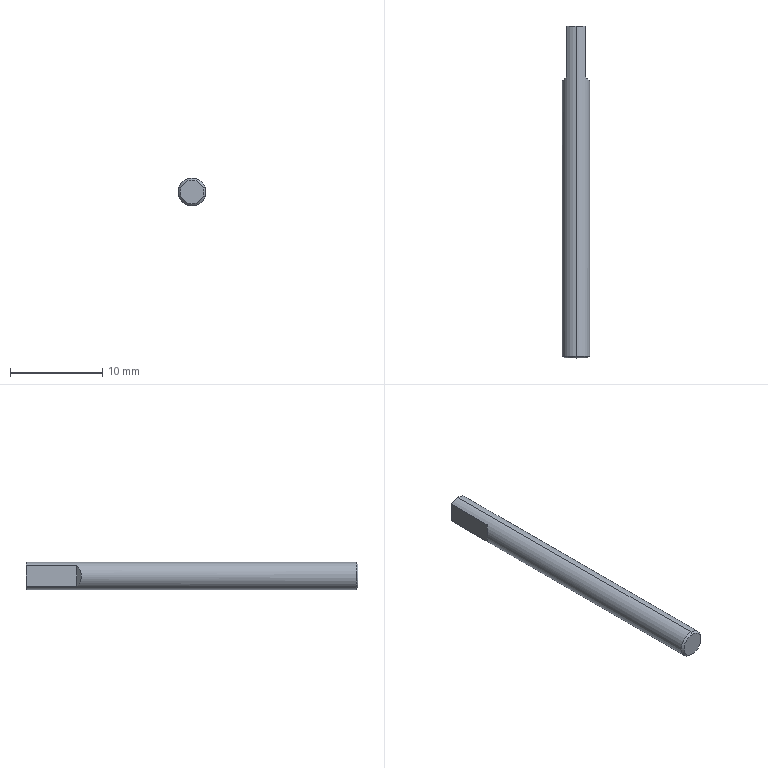Part | SolidWorks | features Chamfer 2, Extrusion 1, ICE 1 | 1 solid | 10 faces | box 3 x 36 x 3 mm | volume 245.456 mm3 | plane 6 | cone 2 | cylinder 2 | commonest cylinder face diameters 3 x2
STEP:
#1=CARTESIAN_POINT('',(0.,0.,-1.3));
#2=VERTEX_POINT('',#1);
#3=CARTESIAN_POINT('',(0.,0.,1.3));
#4=VERTEX_POINT('',#3);
#5=CARTESIAN_POINT('',(0.,0.,0.));
#6=DIRECTION('',(0.,-1.,0.));
#7=DIRECTION('',(0.,0.,1.));
#8=AXIS2_PLACEMENT_3D('',#5,#6,#7);
#9=CIRCLE('',#8,1.3);
#10=EDGE_CURVE('',#2,#4,#9,.T.);
#11=ORIENTED_EDGE('',*,*,#10,.F.);
#12=CARTESIAN_POINT('',(0.,0.2,-1.5));
#13=VERTEX_POINT('',#12);
#14=CARTESIAN_POINT('',(0.,0.2,-1.5));
#15=DIRECTION('',(0.,0.7071,-0.7071));
#16=VECTOR('',#15,1000.);
#17=LINE('',#14,#16);
#18=EDGE_CURVE('',#2,#13,#17,.T.);
#19=ORIENTED_EDGE('',*,*,#18,.T.);
#20=CARTESIAN_POINT('',(0.,0.2,1.5));
#21=VERTEX_POINT('',#20);
#22=CARTESIAN_POINT('',(0.,0.2,0.));
#23=DIRECTION('',(0.,1.,0.));
#24=DIRECTION('',(0.,0.,1.));
#25=AXIS2_PLACEMENT_3D('',#22,#23,#24);
#26=CIRCLE('',#25,1.5);
#27=EDGE_CURVE('',#21,#13,#26,.T.);
#28=ORIENTED_EDGE('',*,*,#27,.F.);
#29=CARTESIAN_POINT('',(0.,0.2,1.5));
#30=DIRECTION('',(0.,0.7071,0.7071));
#31=VECTOR('',#30,1000.);
#32=LINE('',#29,#31);
#33=EDGE_CURVE('',#4,#21,#32,.T.);
#34=ORIENTED_EDGE('',*,*,#33,.F.);
#35=EDGE_LOOP('',(#11,#19,#28,#34));
#36=FACE_OUTER_BOUND('',#35,.T.);
#37=CARTESIAN_POINT('',(0.,0.2,0.));
#38=DIRECTION('',(0.,1.,0.));
#39=DIRECTION('',(0.,0.,1.));
#40=AXIS2_PLACEMENT_3D('',#37,#38,#39);
#41=CONICAL_SURFACE('',#40,1.5,0.7854);
#42=ADVANCED_FACE('',(#36),#41,.T.);
#43=CARTESIAN_POINT('',(0.,36.,1.5));
#44=VERTEX_POINT('',#43);
#45=CARTESIAN_POINT('',(1.,36.,1.118));
#46=VERTEX_POINT('',#45);
#47=CARTESIAN_POINT('',(0.,36.,0.));
#48=DIRECTION('',(0.,1.,0.));
#49=DIRECTION('',(0.,0.,1.));
#50=AXIS2_PLACEMENT_3D('',#47,#48,#49);
#51=CIRCLE('',#50,1.5);
#52=EDGE_CURVE('',#44,#46,#51,.T.);
#53=ORIENTED_EDGE('',*,*,#52,.F.);
#54=CARTESIAN_POINT('',(0.,36.,1.5));
#55=DIRECTION('',(0.,-1.,0.));
#56=VECTOR('',#55,1000.);
#57=LINE('',#54,#56);
#58=EDGE_CURVE('',#44,#21,#57,.T.);
#59=ORIENTED_EDGE('',*,*,#58,.T.);
#60=ORIENTED_EDGE('',*,*,#27,.T.);
#61=CARTESIAN_POINT('',(0.,36.,-1.5));
#62=VERTEX_POINT('',#61);
#63=CARTESIAN_POINT('',(0.,36.,-1.5));
#64=DIRECTION('',(0.,-1.,0.));
#65=VECTOR('',#64,1000.);
#66=LINE('',#63,#65);
#67=EDGE_CURVE('',#62,#13,#66,.T.);
#68=ORIENTED_EDGE('',*,*,#67,.F.);
#69=CARTESIAN_POINT('',(1.,36.,-1.118));
#70=VERTEX_POINT('',#69);
#71=CARTESIAN_POINT('',(0.,36.,0.));
#72=DIRECTION('',(0.,1.,0.));
#73=DIRECTION('',(0.,0.,1.));
#74=AXIS2_PLACEMENT_3D('',#71,#72,#73);
#75=CIRCLE('',#74,1.5);
#76=EDGE_CURVE('',#70,#62,#75,.T.);
#77=ORIENTED_EDGE('',*,*,#76,.F.);
#78=CARTESIAN_POINT('',(1.,30.5,-1.118));
#79=VERTEX_POINT('',#78);
#80=CARTESIAN_POINT('',(1.,36.,-1.118));
#81=DIRECTION('',(0.,1.,0.));
#82=VECTOR('',#81,1000.);
#83=LINE('',#80,#82);
#84=EDGE_CURVE('',#79,#70,#83,.T.);
#85=ORIENTED_EDGE('',*,*,#84,.F.);
#86=CARTESIAN_POINT('',(1.,30.5,1.118));
#87=VERTEX_POINT('',#86);
#88=CARTESIAN_POINT('',(1.,30.5,-1.118));
#89=CARTESIAN_POINT('',(1.714,29.786,-0.4792));
#90=CARTESIAN_POINT('',(1.714,29.786,0.4792));
#91=CARTESIAN_POINT('',(1.,30.5,1.118));
#92=(BOUNDED_CURVE()B_SPLINE_CURVE(3,(#88,#89,#90,#91),.UNSPECIFIED.,.F.,.F.)B_SPLINE_CURVE_WITH_KNOTS((4,4),(5.442,7.124),.UNSPECIFIED.)CURVE()GEOMETRIC_REPRESENTATION_ITEM()RATIONAL_B_SPLINE_CURVE((1.,0.7778,0.7778,1.))REPRESENTATION_ITEM(''));
#93=EDGE_CURVE('',#79,#87,#92,.T.);
#94=ORIENTED_EDGE('',*,*,#93,.T.);
#95=CARTESIAN_POINT('',(1.,36.,1.118));
#96=DIRECTION('',(0.,-1.,0.));
#97=VECTOR('',#96,1000.);
#98=LINE('',#95,#97);
#99=EDGE_CURVE('',#46,#87,#98,.T.);
#100=ORIENTED_EDGE('',*,*,#99,.F.);
#101=EDGE_LOOP('',(#53,#59,#60,#68,#77,#85,#94,#100));
#102=FACE_OUTER_BOUND('',#101,.T.);
#103=CARTESIAN_POINT('',(0.,36.,0.));
#104=DIRECTION('',(0.,-1.,0.));
#105=DIRECTION('',(0.,0.,-1.));
#106=AXIS2_PLACEMENT_3D('',#103,#104,#105);
#107=CYLINDRICAL_SURFACE('',#106,1.5);
#108=ADVANCED_FACE('',(#102),#107,.T.);
#109=ORIENTED_EDGE('',*,*,#58,.F.);
#110=CARTESIAN_POINT('',(-1.,36.,1.118));
#111=VERTEX_POINT('',#110);
#112=CARTESIAN_POINT('',(0.,36.,0.));
#113=DIRECTION('',(0.,1.,0.));
#114=DIRECTION('',(0.,0.,1.));
#115=AXIS2_PLACEMENT_3D('',#112,#113,#114);
#116=CIRCLE('',#115,1.5);
#117=EDGE_CURVE('',#111,#44,#116,.T.);
#118=ORIENTED_EDGE('',*,*,#117,.F.);
#119=CARTESIAN_POINT('',(-1.,30.5,1.118));
#120=VERTEX_POINT('',#119);
#121=CARTESIAN_POINT('',(-1.,36.,1.118));
#122=DIRECTION('',(0.,1.,0.));
#123=VECTOR('',#122,1000.);
#124=LINE('',#121,#123);
#125=EDGE_CURVE('',#120,#111,#124,.T.);
#126=ORIENTED_EDGE('',*,*,#125,.F.);
#127=CARTESIAN_POINT('',(-1.,30.5,-1.118));
#128=VERTEX_POINT('',#127);
#129=CARTESIAN_POINT('',(-1.,30.5,1.118));
#130=CARTESIAN_POINT('',(-1.714,29.786,0.4792));
#131=CARTESIAN_POINT('',(-1.714,29.786,-0.4792));
#132=CARTESIAN_POINT('',(-1.,30.5,-1.118));
#133=(BOUNDED_CURVE()B_SPLINE_CURVE(3,(#129,#130,#131,#132),.UNSPECIFIED.,.F.,.T.)B_SPLINE_CURVE_WITH_KNOTS((4,4),(5.442,7.124),.UNSPECIFIED.)CURVE()GEOMETRIC_REPRESENTATION_ITEM()RATIONAL_B_SPLINE_CURVE((1.,0.7778,0.7778,1.))REPRESENTATION_ITEM(''));
#134=EDGE_CURVE('',#120,#128,#133,.T.);
#135=ORIENTED_EDGE('',*,*,#134,.T.);
#136=CARTESIAN_POINT('',(-1.,36.,-1.118));
#137=VERTEX_POINT('',#136);
#138=CARTESIAN_POINT('',(-1.,36.,-1.118));
#139=DIRECTION('',(0.,-1.,0.));
#140=VECTOR('',#139,1000.);
#141=LINE('',#138,#140);
#142=EDGE_CURVE('',#137,#128,#141,.T.);
#143=ORIENTED_EDGE('',*,*,#142,.F.);
#144=CARTESIAN_POINT('',(0.,36.,0.));
#145=DIRECTION('',(0.,1.,0.));
#146=DIRECTION('',(0.,0.,1.));
#147=AXIS2_PLACEMENT_3D('',#144,#145,#146);
#148=CIRCLE('',#147,1.5);
#149=EDGE_CURVE('',#62,#137,#148,.T.);
#150=ORIENTED_EDGE('',*,*,#149,.F.);
#151=ORIENTED_EDGE('',*,*,#67,.T.);
#152=CARTESIAN_POINT('',(0.,0.2,0.));
#153=DIRECTION('',(0.,1.,0.));
#154=DIRECTION('',(0.,0.,1.));
#155=AXIS2_PLACEMENT_3D('',#152,#153,#154);
#156=CIRCLE('',#155,1.5);
#157=EDGE_CURVE('',#13,#21,#156,.T.);
#158=ORIENTED_EDGE('',*,*,#157,.T.);
#159=EDGE_LOOP('',(#109,#118,#126,#135,#143,#150,#151,#158));
#160=FACE_OUTER_BOUND('',#159,.T.);
#161=CARTESIAN_POINT('',(0.,36.,0.));
#162=DIRECTION('',(0.,-1.,0.));
#163=DIRECTION('',(0.,0.,-1.));
#164=AXIS2_PLACEMENT_3D('',#161,#162,#163);
#165=CYLINDRICAL_SURFACE('',#164,1.5);
#166=ADVANCED_FACE('',(#160),#165,.T.);
#167=ORIENTED_EDGE('',*,*,#117,.T.);
#168=ORIENTED_EDGE('',*,*,#52,.T.);
#169=CARTESIAN_POINT('',(1.,36.,0.));
#170=DIRECTION('',(0.,0.,-1.));
#171=VECTOR('',#170,1000.);
#172=LINE('',#169,#171);
#173=EDGE_CURVE('',#46,#70,#172,.T.);
#174=ORIENTED_EDGE('',*,*,#173,.T.);
#175=ORIENTED_EDGE('',*,*,#76,.T.);
#176=ORIENTED_EDGE('',*,*,#149,.T.);
#177=CARTESIAN_POINT('',(-1.,36.,0.));
#178=DIRECTION('',(0.,0.,1.));
#179=VECTOR('',#178,1000.);
#180=LINE('',#177,#179);
#181=EDGE_CURVE('',#137,#111,#180,.T.);
#182=ORIENTED_EDGE('',*,*,#181,.T.);
#183=EDGE_LOOP('',(#167,#168,#174,#175,#176,#182));
#184=FACE_OUTER_BOUND('',#183,.T.);
#185=CARTESIAN_POINT('',(0.,36.,0.));
#186=DIRECTION('',(0.,1.,0.));
#187=DIRECTION('',(0.,0.,1.));
#188=AXIS2_PLACEMENT_3D('',#185,#186,#187);
#189=PLANE('',#188);
#190=ADVANCED_FACE('',(#184),#189,.T.);
#191=CARTESIAN_POINT('',(0.,0.,0.));
#192=DIRECTION('',(0.,-1.,0.));
#193=DIRECTION('',(0.,0.,1.));
#194=AXIS2_PLACEMENT_3D('',#191,#192,#193);
#195=CIRCLE('',#194,1.3);
#196=EDGE_CURVE('',#4,#2,#195,.T.);
#197=ORIENTED_EDGE('',*,*,#196,.T.);
#198=ORIENTED_EDGE('',*,*,#10,.T.);
#199=EDGE_LOOP('',(#197,#198));
#200=FACE_OUTER_BOUND('',#199,.T.);
#201=CARTESIAN_POINT('',(0.,0.,0.));
#202=DIRECTION('',(0.,1.,0.));
#203=DIRECTION('',(0.,0.,1.));
#204=AXIS2_PLACEMENT_3D('',#201,#202,#203);
#205=PLANE('',#204);
#206=ADVANCED_FACE('',(#200),#205,.F.);
#207=ORIENTED_EDGE('',*,*,#18,.F.);
#208=ORIENTED_EDGE('',*,*,#196,.F.);
#209=ORIENTED_EDGE('',*,*,#33,.T.);
#210=ORIENTED_EDGE('',*,*,#157,.F.);
#211=EDGE_LOOP('',(#207,#208,#209,#210));
#212=FACE_OUTER_BOUND('',#211,.T.);
#213=CARTESIAN_POINT('',(0.,0.2,0.));
#214=DIRECTION('',(0.,1.,0.));
#215=DIRECTION('',(0.,0.,1.));
#216=AXIS2_PLACEMENT_3D('',#213,#214,#215);
#217=CONICAL_SURFACE('',#216,1.5,0.7854);
#218=ADVANCED_FACE('',(#212),#217,.T.);
#219=ORIENTED_EDGE('',*,*,#142,.T.);
#220=CARTESIAN_POINT('',(-1.,30.5,1.118));
#221=DIRECTION('',(0.,0.,1.));
#222=VECTOR('',#221,1000.);
#223=LINE('',#220,#222);
#224=EDGE_CURVE('',#128,#120,#223,.T.);
#225=ORIENTED_EDGE('',*,*,#224,.T.);
#226=ORIENTED_EDGE('',*,*,#125,.T.);
#227=ORIENTED_EDGE('',*,*,#181,.F.);
#228=EDGE_LOOP('',(#219,#225,#226,#227));
#229=FACE_OUTER_BOUND('',#228,.T.);
#230=CARTESIAN_POINT('',(-1.,30.,-2.));
#231=DIRECTION('',(-1.,0.,0.));
#232=DIRECTION('',(0.,0.,1.));
#233=AXIS2_PLACEMENT_3D('',#230,#231,#232);
#234=PLANE('',#233);
#235=ADVANCED_FACE('',(#229),#234,.T.);
#236=ORIENTED_EDGE('',*,*,#99,.T.);
#237=CARTESIAN_POINT('',(1.,30.5,-1.118));
#238=DIRECTION('',(0.,0.,-1.));
#239=VECTOR('',#238,1000.);
#240=LINE('',#237,#239);
#241=EDGE_CURVE('',#87,#79,#240,.T.);
#242=ORIENTED_EDGE('',*,*,#241,.T.);
#243=ORIENTED_EDGE('',*,*,#84,.T.);
#244=ORIENTED_EDGE('',*,*,#173,.F.);
#245=EDGE_LOOP('',(#236,#242,#243,#244));
#246=FACE_OUTER_BOUND('',#245,.T.);
#247=CARTESIAN_POINT('',(1.,30.,-2.));
#248=DIRECTION('',(1.,0.,0.));
#249=DIRECTION('',(0.,0.,-1.));
#250=AXIS2_PLACEMENT_3D('',#247,#248,#249);
#251=PLANE('',#250);
#252=ADVANCED_FACE('',(#246),#251,.T.);
#253=ORIENTED_EDGE('',*,*,#241,.F.);
#254=ORIENTED_EDGE('',*,*,#93,.F.);
#255=EDGE_LOOP('',(#253,#254));
#256=FACE_OUTER_BOUND('',#255,.T.);
#257=CARTESIAN_POINT('',(1.,30.5,-2.));
#258=DIRECTION('',(0.7071,0.7071,0.));
#259=DIRECTION('',(0.,0.,1.));
#260=AXIS2_PLACEMENT_3D('',#257,#258,#259);
#261=PLANE('',#260);
#262=ADVANCED_FACE('',(#256),#261,.T.);
#263=ORIENTED_EDGE('',*,*,#224,.F.);
#264=ORIENTED_EDGE('',*,*,#134,.F.);
#265=EDGE_LOOP('',(#263,#264));
#266=FACE_OUTER_BOUND('',#265,.T.);
#267=CARTESIAN_POINT('',(-1.,30.5,-2.));
#268=DIRECTION('',(-0.7071,0.7071,0.));
#269=DIRECTION('',(0.,0.,-1.));
#270=AXIS2_PLACEMENT_3D('',#267,#268,#269);
#271=PLANE('',#270);
#272=ADVANCED_FACE('',(#266),#271,.T.);
#273=CLOSED_SHELL('',(#42,#108,#166,#190,#206,#218,#235,#252,#262,#272));
#274=MANIFOLD_SOLID_BREP('',#273);
#275=CARTESIAN_POINT('',(0.,0.,0.));
#276=DIRECTION('',(0.,0.,1.));
#277=DIRECTION('',(1.,0.,0.));
#278=AXIS2_PLACEMENT_3D('',#275,#276,#277);
#279=(LENGTH_UNIT()NAMED_UNIT(*)SI_UNIT(.MILLI.,.METRE.));
#280=UNCERTAINTY_MEASURE_WITH_UNIT(LENGTH_MEASURE(0.00001),#279,'','');
#281=(NAMED_UNIT(*)PLANE_ANGLE_UNIT()SI_UNIT($,.RADIAN.));
#282=(NAMED_UNIT(*)SI_UNIT($,.STERADIAN.)SOLID_ANGLE_UNIT());
#283=(GEOMETRIC_REPRESENTATION_CONTEXT(3)GLOBAL_UNCERTAINTY_ASSIGNED_CONTEXT((#280))GLOBAL_UNIT_ASSIGNED_CONTEXT((#279,#281,#282))REPRESENTATION_CONTEXT('',''));
#284=ADVANCED_BREP_SHAPE_REPRESENTATION('',(#274,#278),#283);